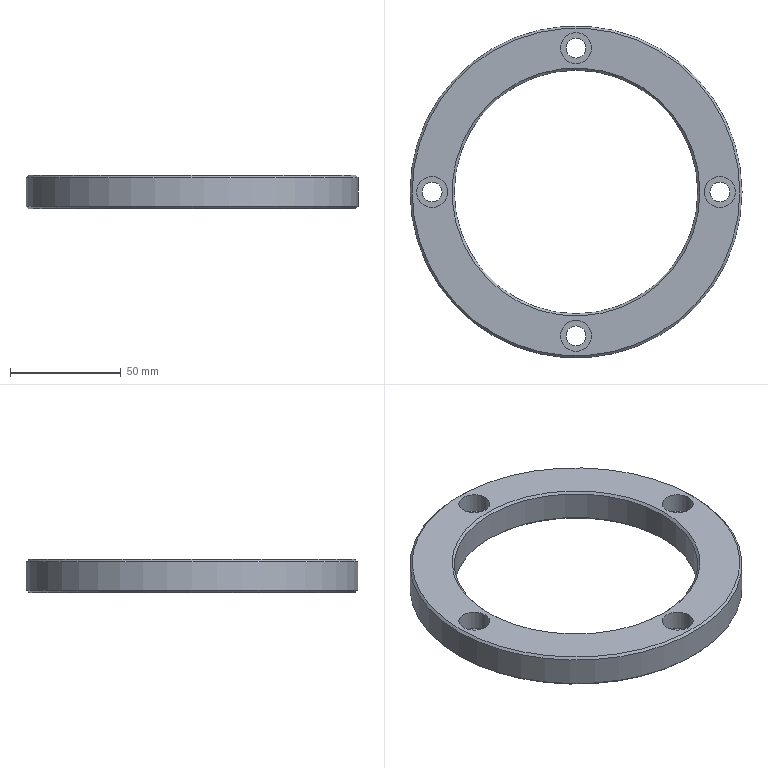Part | STEP file | solid 68 | 1 solid | 20 faces | box 150 x 150 x 15 mm | volume 114637 mm3 | cylinder 10 | plane 6 | cone 4 | commonest cylinder face diameters 9 x4 14 x4 110 x1 150 x1